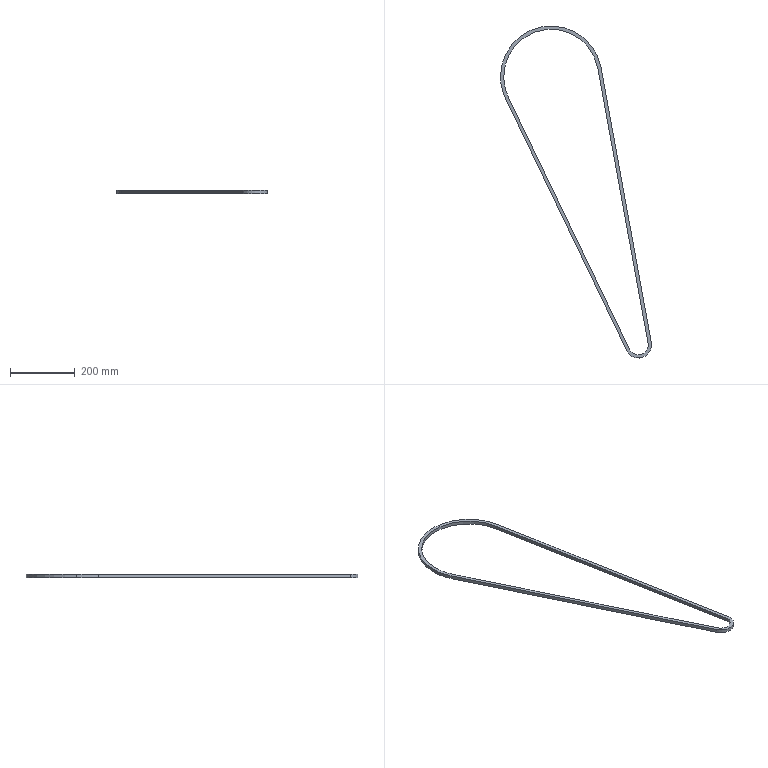Part | SolidWorks | features ExtruThin 1 | 1 solid | 12 faces | box 465.093 x 1023 x 10 mm | volume 233862 mm3 | cylinder 6 | plane 6 | commonest cylinder face diameters 292.108 x2 312.108 x2 60.38 x1 80.38 x1
STEP:
#1=CARTESIAN_POINT('',(143.673,109.871,10.));
#2=VERTEX_POINT('',#1);
#3=CARTESIAN_POINT('',(-146.054,83.608,10.));
#4=VERTEX_POINT('',#3);
#5=CARTESIAN_POINT('',(0.,83.608,10.));
#6=DIRECTION('',(0.,0.,1.));
#7=DIRECTION('',(1.,0.,0.));
#8=AXIS2_PLACEMENT_3D('',#5,#6,#7);
#9=CIRCLE('',#8,146.054);
#10=EDGE_CURVE('',#2,#4,#9,.T.);
#11=ORIENTED_EDGE('',*,*,#10,.T.);
#12=CARTESIAN_POINT('',(-146.054,83.608,0.));
#13=VERTEX_POINT('',#12);
#14=CARTESIAN_POINT('',(-146.054,83.608,10.));
#15=DIRECTION('',(0.,0.,-1.));
#16=VECTOR('',#15,1000.);
#17=LINE('',#14,#16);
#18=EDGE_CURVE('',#4,#13,#17,.T.);
#19=ORIENTED_EDGE('',*,*,#18,.T.);
#20=CARTESIAN_POINT('',(143.673,109.871,0.));
#21=VERTEX_POINT('',#20);
#22=CARTESIAN_POINT('',(0.,83.608,0.));
#23=DIRECTION('',(0.,0.,1.));
#24=DIRECTION('',(1.,0.,0.));
#25=AXIS2_PLACEMENT_3D('',#22,#23,#24);
#26=CIRCLE('',#25,146.054);
#27=EDGE_CURVE('',#21,#13,#26,.T.);
#28=ORIENTED_EDGE('',*,*,#27,.F.);
#29=CARTESIAN_POINT('',(143.673,109.871,10.));
#30=DIRECTION('',(0.,0.,-1.));
#31=VECTOR('',#30,1000.);
#32=LINE('',#29,#31);
#33=EDGE_CURVE('',#2,#21,#32,.T.);
#34=ORIENTED_EDGE('',*,*,#33,.F.);
#35=EDGE_LOOP('',(#11,#19,#28,#34));
#36=FACE_OUTER_BOUND('',#35,.T.);
#37=CARTESIAN_POINT('',(0.,83.608,10.));
#38=DIRECTION('',(0.,0.,-1.));
#39=DIRECTION('',(-1.,0.,0.));
#40=AXIS2_PLACEMENT_3D('',#37,#38,#39);
#41=CYLINDRICAL_SURFACE('',#40,146.054);
#42=ADVANCED_FACE('',(#36),#41,.F.);
#43=CARTESIAN_POINT('',(-156.054,83.608,10.));
#44=VERTEX_POINT('',#43);
#45=CARTESIAN_POINT('',(-140.636,15.975,10.));
#46=VERTEX_POINT('',#45);
#47=CARTESIAN_POINT('',(0.,83.608,10.));
#48=DIRECTION('',(0.,0.,1.));
#49=DIRECTION('',(1.,0.,0.));
#50=AXIS2_PLACEMENT_3D('',#47,#48,#49);
#51=CIRCLE('',#50,156.054);
#52=EDGE_CURVE('',#44,#46,#51,.T.);
#53=ORIENTED_EDGE('',*,*,#52,.F.);
#54=CARTESIAN_POINT('',(-156.054,83.608,0.));
#55=VERTEX_POINT('',#54);
#56=CARTESIAN_POINT('',(-156.054,83.608,10.));
#57=DIRECTION('',(0.,0.,-1.));
#58=VECTOR('',#57,1000.);
#59=LINE('',#56,#58);
#60=EDGE_CURVE('',#44,#55,#59,.T.);
#61=ORIENTED_EDGE('',*,*,#60,.T.);
#62=CARTESIAN_POINT('',(-140.636,15.975,0.));
#63=VERTEX_POINT('',#62);
#64=CARTESIAN_POINT('',(0.,83.608,0.));
#65=DIRECTION('',(0.,0.,1.));
#66=DIRECTION('',(1.,0.,0.));
#67=AXIS2_PLACEMENT_3D('',#64,#65,#66);
#68=CIRCLE('',#67,156.054);
#69=EDGE_CURVE('',#55,#63,#68,.T.);
#70=ORIENTED_EDGE('',*,*,#69,.T.);
#71=CARTESIAN_POINT('',(-140.636,15.975,10.));
#72=DIRECTION('',(0.,0.,-1.));
#73=VECTOR('',#72,1000.);
#74=LINE('',#71,#73);
#75=EDGE_CURVE('',#46,#63,#74,.T.);
#76=ORIENTED_EDGE('',*,*,#75,.F.);
#77=EDGE_LOOP('',(#53,#61,#70,#76));
#78=FACE_OUTER_BOUND('',#77,.T.);
#79=CARTESIAN_POINT('',(0.,83.608,10.));
#80=DIRECTION('',(0.,0.,-1.));
#81=DIRECTION('',(-1.,0.,0.));
#82=AXIS2_PLACEMENT_3D('',#79,#80,#81);
#83=CYLINDRICAL_SURFACE('',#82,156.054);
#84=ADVANCED_FACE('',(#78),#83,.T.);
#85=CARTESIAN_POINT('',(232.63,-760.201,10.));
#86=VERTEX_POINT('',#85);
#87=CARTESIAN_POINT('',(308.384,-735.556,10.));
#88=VERTEX_POINT('',#87);
#89=CARTESIAN_POINT('',(268.849,-742.783,10.));
#90=DIRECTION('',(0.,0.,1.));
#91=DIRECTION('',(1.,0.,0.));
#92=AXIS2_PLACEMENT_3D('',#89,#90,#91);
#93=CIRCLE('',#92,40.19);
#94=EDGE_CURVE('',#86,#88,#93,.T.);
#95=ORIENTED_EDGE('',*,*,#94,.T.);
#96=CARTESIAN_POINT('',(153.51,111.669,10.));
#97=VERTEX_POINT('',#96);
#98=CARTESIAN_POINT('',(153.51,111.669,10.));
#99=DIRECTION('',(-0.1798,0.9837,0.));
#100=VECTOR('',#99,1000.);
#101=LINE('',#98,#100);
#102=EDGE_CURVE('',#88,#97,#101,.T.);
#103=ORIENTED_EDGE('',*,*,#102,.T.);
#104=CARTESIAN_POINT('',(0.,83.608,10.));
#105=DIRECTION('',(0.,0.,1.));
#106=DIRECTION('',(1.,0.,0.));
#107=AXIS2_PLACEMENT_3D('',#104,#105,#106);
#108=CIRCLE('',#107,156.054);
#109=EDGE_CURVE('',#97,#44,#108,.T.);
#110=ORIENTED_EDGE('',*,*,#109,.T.);
#111=ORIENTED_EDGE('',*,*,#52,.T.);
#112=CARTESIAN_POINT('',(-140.636,15.975,10.));
#113=DIRECTION('',(0.4334,-0.9012,0.));
#114=VECTOR('',#113,1000.);
#115=LINE('',#112,#114);
#116=EDGE_CURVE('',#46,#86,#115,.T.);
#117=ORIENTED_EDGE('',*,*,#116,.T.);
#118=EDGE_LOOP('',(#95,#103,#110,#111,#117));
#119=FACE_OUTER_BOUND('',#118,.T.);
#120=CARTESIAN_POINT('',(298.547,-737.354,10.));
#121=VERTEX_POINT('',#120);
#122=CARTESIAN_POINT('',(143.673,109.871,10.));
#123=DIRECTION('',(-0.1798,0.9837,0.));
#124=VECTOR('',#123,1000.);
#125=LINE('',#122,#124);
#126=EDGE_CURVE('',#121,#2,#125,.T.);
#127=ORIENTED_EDGE('',*,*,#126,.F.);
#128=CARTESIAN_POINT('',(241.642,-755.867,10.));
#129=VERTEX_POINT('',#128);
#130=CARTESIAN_POINT('',(268.849,-742.783,10.));
#131=DIRECTION('',(0.,0.,1.));
#132=DIRECTION('',(1.,0.,0.));
#133=AXIS2_PLACEMENT_3D('',#130,#131,#132);
#134=CIRCLE('',#133,30.19);
#135=EDGE_CURVE('',#129,#121,#134,.T.);
#136=ORIENTED_EDGE('',*,*,#135,.F.);
#137=CARTESIAN_POINT('',(-131.624,20.309,10.));
#138=VERTEX_POINT('',#137);
#139=CARTESIAN_POINT('',(-131.624,20.309,10.));
#140=DIRECTION('',(0.4334,-0.9012,0.));
#141=VECTOR('',#140,1000.);
#142=LINE('',#139,#141);
#143=EDGE_CURVE('',#138,#129,#142,.T.);
#144=ORIENTED_EDGE('',*,*,#143,.F.);
#145=CARTESIAN_POINT('',(0.,83.608,10.));
#146=DIRECTION('',(0.,0.,1.));
#147=DIRECTION('',(1.,0.,0.));
#148=AXIS2_PLACEMENT_3D('',#145,#146,#147);
#149=CIRCLE('',#148,146.054);
#150=EDGE_CURVE('',#4,#138,#149,.T.);
#151=ORIENTED_EDGE('',*,*,#150,.F.);
#152=ORIENTED_EDGE('',*,*,#10,.F.);
#153=EDGE_LOOP('',(#127,#136,#144,#151,#152));
#154=FACE_BOUND('',#153,.T.);
#155=CARTESIAN_POINT('',(268.849,-742.783,10.));
#156=DIRECTION('',(0.,0.,1.));
#157=DIRECTION('',(1.,0.,0.));
#158=AXIS2_PLACEMENT_3D('',#155,#156,#157);
#159=PLANE('',#158);
#160=ADVANCED_FACE('',(#119,#154),#159,.T.);
#161=CARTESIAN_POINT('',(232.63,-760.201,0.));
#162=VERTEX_POINT('',#161);
#163=CARTESIAN_POINT('',(308.384,-735.556,0.));
#164=VERTEX_POINT('',#163);
#165=CARTESIAN_POINT('',(268.849,-742.783,0.));
#166=DIRECTION('',(0.,0.,1.));
#167=DIRECTION('',(1.,0.,0.));
#168=AXIS2_PLACEMENT_3D('',#165,#166,#167);
#169=CIRCLE('',#168,40.19);
#170=EDGE_CURVE('',#162,#164,#169,.T.);
#171=ORIENTED_EDGE('',*,*,#170,.F.);
#172=CARTESIAN_POINT('',(-140.636,15.975,0.));
#173=DIRECTION('',(0.4334,-0.9012,0.));
#174=VECTOR('',#173,1000.);
#175=LINE('',#172,#174);
#176=EDGE_CURVE('',#63,#162,#175,.T.);
#177=ORIENTED_EDGE('',*,*,#176,.F.);
#178=ORIENTED_EDGE('',*,*,#69,.F.);
#179=CARTESIAN_POINT('',(153.51,111.669,0.));
#180=VERTEX_POINT('',#179);
#181=CARTESIAN_POINT('',(0.,83.608,0.));
#182=DIRECTION('',(0.,0.,1.));
#183=DIRECTION('',(1.,0.,0.));
#184=AXIS2_PLACEMENT_3D('',#181,#182,#183);
#185=CIRCLE('',#184,156.054);
#186=EDGE_CURVE('',#180,#55,#185,.T.);
#187=ORIENTED_EDGE('',*,*,#186,.F.);
#188=CARTESIAN_POINT('',(153.51,111.669,0.));
#189=DIRECTION('',(-0.1798,0.9837,0.));
#190=VECTOR('',#189,1000.);
#191=LINE('',#188,#190);
#192=EDGE_CURVE('',#164,#180,#191,.T.);
#193=ORIENTED_EDGE('',*,*,#192,.F.);
#194=EDGE_LOOP('',(#171,#177,#178,#187,#193));
#195=FACE_OUTER_BOUND('',#194,.T.);
#196=CARTESIAN_POINT('',(241.642,-755.867,0.));
#197=VERTEX_POINT('',#196);
#198=CARTESIAN_POINT('',(298.547,-737.354,0.));
#199=VERTEX_POINT('',#198);
#200=CARTESIAN_POINT('',(268.849,-742.783,0.));
#201=DIRECTION('',(0.,0.,1.));
#202=DIRECTION('',(1.,0.,0.));
#203=AXIS2_PLACEMENT_3D('',#200,#201,#202);
#204=CIRCLE('',#203,30.19);
#205=EDGE_CURVE('',#197,#199,#204,.T.);
#206=ORIENTED_EDGE('',*,*,#205,.T.);
#207=CARTESIAN_POINT('',(143.673,109.871,0.));
#208=DIRECTION('',(-0.1798,0.9837,0.));
#209=VECTOR('',#208,1000.);
#210=LINE('',#207,#209);
#211=EDGE_CURVE('',#199,#21,#210,.T.);
#212=ORIENTED_EDGE('',*,*,#211,.T.);
#213=ORIENTED_EDGE('',*,*,#27,.T.);
#214=CARTESIAN_POINT('',(-131.624,20.309,0.));
#215=VERTEX_POINT('',#214);
#216=CARTESIAN_POINT('',(0.,83.608,0.));
#217=DIRECTION('',(0.,0.,1.));
#218=DIRECTION('',(1.,0.,0.));
#219=AXIS2_PLACEMENT_3D('',#216,#217,#218);
#220=CIRCLE('',#219,146.054);
#221=EDGE_CURVE('',#13,#215,#220,.T.);
#222=ORIENTED_EDGE('',*,*,#221,.T.);
#223=CARTESIAN_POINT('',(-131.624,20.309,0.));
#224=DIRECTION('',(0.4334,-0.9012,0.));
#225=VECTOR('',#224,1000.);
#226=LINE('',#223,#225);
#227=EDGE_CURVE('',#215,#197,#226,.T.);
#228=ORIENTED_EDGE('',*,*,#227,.T.);
#229=EDGE_LOOP('',(#206,#212,#213,#222,#228));
#230=FACE_BOUND('',#229,.T.);
#231=CARTESIAN_POINT('',(268.849,-742.783,0.));
#232=DIRECTION('',(0.,0.,1.));
#233=DIRECTION('',(1.,0.,0.));
#234=AXIS2_PLACEMENT_3D('',#231,#232,#233);
#235=PLANE('',#234);
#236=ADVANCED_FACE('',(#195,#230),#235,.F.);
#237=ORIENTED_EDGE('',*,*,#170,.T.);
#238=CARTESIAN_POINT('',(308.384,-735.556,10.));
#239=DIRECTION('',(0.,0.,-1.));
#240=VECTOR('',#239,1000.);
#241=LINE('',#238,#240);
#242=EDGE_CURVE('',#88,#164,#241,.T.);
#243=ORIENTED_EDGE('',*,*,#242,.F.);
#244=ORIENTED_EDGE('',*,*,#94,.F.);
#245=CARTESIAN_POINT('',(232.63,-760.201,10.));
#246=DIRECTION('',(0.,0.,-1.));
#247=VECTOR('',#246,1000.);
#248=LINE('',#245,#247);
#249=EDGE_CURVE('',#86,#162,#248,.T.);
#250=ORIENTED_EDGE('',*,*,#249,.T.);
#251=EDGE_LOOP('',(#237,#243,#244,#250));
#252=FACE_OUTER_BOUND('',#251,.T.);
#253=CARTESIAN_POINT('',(268.849,-742.783,10.));
#254=DIRECTION('',(0.,0.,-1.));
#255=DIRECTION('',(-1.,0.,0.));
#256=AXIS2_PLACEMENT_3D('',#253,#254,#255);
#257=CYLINDRICAL_SURFACE('',#256,40.19);
#258=ADVANCED_FACE('',(#252),#257,.T.);
#259=ORIENTED_EDGE('',*,*,#192,.T.);
#260=CARTESIAN_POINT('',(153.51,111.669,10.));
#261=DIRECTION('',(0.,0.,-1.));
#262=VECTOR('',#261,1000.);
#263=LINE('',#260,#262);
#264=EDGE_CURVE('',#97,#180,#263,.T.);
#265=ORIENTED_EDGE('',*,*,#264,.F.);
#266=ORIENTED_EDGE('',*,*,#102,.F.);
#267=ORIENTED_EDGE('',*,*,#242,.T.);
#268=EDGE_LOOP('',(#259,#265,#266,#267));
#269=FACE_OUTER_BOUND('',#268,.T.);
#270=CARTESIAN_POINT('',(153.51,111.669,10.));
#271=DIRECTION('',(-0.9837,-0.1798,0.));
#272=DIRECTION('',(0.1798,-0.9837,0.));
#273=AXIS2_PLACEMENT_3D('',#270,#271,#272);
#274=PLANE('',#273);
#275=ADVANCED_FACE('',(#269),#274,.F.);
#276=ORIENTED_EDGE('',*,*,#60,.F.);
#277=ORIENTED_EDGE('',*,*,#109,.F.);
#278=ORIENTED_EDGE('',*,*,#264,.T.);
#279=ORIENTED_EDGE('',*,*,#186,.T.);
#280=EDGE_LOOP('',(#276,#277,#278,#279));
#281=FACE_OUTER_BOUND('',#280,.T.);
#282=CARTESIAN_POINT('',(0.,83.608,10.));
#283=DIRECTION('',(0.,0.,-1.));
#284=DIRECTION('',(-1.,0.,0.));
#285=AXIS2_PLACEMENT_3D('',#282,#283,#284);
#286=CYLINDRICAL_SURFACE('',#285,156.054);
#287=ADVANCED_FACE('',(#281),#286,.T.);
#288=ORIENTED_EDGE('',*,*,#176,.T.);
#289=ORIENTED_EDGE('',*,*,#249,.F.);
#290=ORIENTED_EDGE('',*,*,#116,.F.);
#291=ORIENTED_EDGE('',*,*,#75,.T.);
#292=EDGE_LOOP('',(#288,#289,#290,#291));
#293=FACE_OUTER_BOUND('',#292,.T.);
#294=CARTESIAN_POINT('',(-140.636,15.975,10.));
#295=DIRECTION('',(0.9012,0.4334,0.));
#296=DIRECTION('',(-0.4334,0.9012,0.));
#297=AXIS2_PLACEMENT_3D('',#294,#295,#296);
#298=PLANE('',#297);
#299=ADVANCED_FACE('',(#293),#298,.F.);
#300=ORIENTED_EDGE('',*,*,#205,.F.);
#301=CARTESIAN_POINT('',(241.642,-755.867,10.));
#302=DIRECTION('',(0.,0.,-1.));
#303=VECTOR('',#302,1000.);
#304=LINE('',#301,#303);
#305=EDGE_CURVE('',#129,#197,#304,.T.);
#306=ORIENTED_EDGE('',*,*,#305,.F.);
#307=ORIENTED_EDGE('',*,*,#135,.T.);
#308=CARTESIAN_POINT('',(298.547,-737.354,10.));
#309=DIRECTION('',(0.,0.,-1.));
#310=VECTOR('',#309,1000.);
#311=LINE('',#308,#310);
#312=EDGE_CURVE('',#121,#199,#311,.T.);
#313=ORIENTED_EDGE('',*,*,#312,.T.);
#314=EDGE_LOOP('',(#300,#306,#307,#313));
#315=FACE_OUTER_BOUND('',#314,.T.);
#316=CARTESIAN_POINT('',(268.849,-742.783,10.));
#317=DIRECTION('',(0.,0.,-1.));
#318=DIRECTION('',(-1.,0.,0.));
#319=AXIS2_PLACEMENT_3D('',#316,#317,#318);
#320=CYLINDRICAL_SURFACE('',#319,30.19);
#321=ADVANCED_FACE('',(#315),#320,.F.);
#322=ORIENTED_EDGE('',*,*,#211,.F.);
#323=ORIENTED_EDGE('',*,*,#312,.F.);
#324=ORIENTED_EDGE('',*,*,#126,.T.);
#325=ORIENTED_EDGE('',*,*,#33,.T.);
#326=EDGE_LOOP('',(#322,#323,#324,#325));
#327=FACE_OUTER_BOUND('',#326,.T.);
#328=CARTESIAN_POINT('',(143.673,109.871,10.));
#329=DIRECTION('',(-0.9837,-0.1798,0.));
#330=DIRECTION('',(0.1798,-0.9837,0.));
#331=AXIS2_PLACEMENT_3D('',#328,#329,#330);
#332=PLANE('',#331);
#333=ADVANCED_FACE('',(#327),#332,.T.);
#334=ORIENTED_EDGE('',*,*,#18,.F.);
#335=ORIENTED_EDGE('',*,*,#150,.T.);
#336=CARTESIAN_POINT('',(-131.624,20.309,10.));
#337=DIRECTION('',(0.,0.,-1.));
#338=VECTOR('',#337,1000.);
#339=LINE('',#336,#338);
#340=EDGE_CURVE('',#138,#215,#339,.T.);
#341=ORIENTED_EDGE('',*,*,#340,.T.);
#342=ORIENTED_EDGE('',*,*,#221,.F.);
#343=EDGE_LOOP('',(#334,#335,#341,#342));
#344=FACE_OUTER_BOUND('',#343,.T.);
#345=CARTESIAN_POINT('',(0.,83.608,10.));
#346=DIRECTION('',(0.,0.,-1.));
#347=DIRECTION('',(-1.,0.,0.));
#348=AXIS2_PLACEMENT_3D('',#345,#346,#347);
#349=CYLINDRICAL_SURFACE('',#348,146.054);
#350=ADVANCED_FACE('',(#344),#349,.F.);
#351=ORIENTED_EDGE('',*,*,#227,.F.);
#352=ORIENTED_EDGE('',*,*,#340,.F.);
#353=ORIENTED_EDGE('',*,*,#143,.T.);
#354=ORIENTED_EDGE('',*,*,#305,.T.);
#355=EDGE_LOOP('',(#351,#352,#353,#354));
#356=FACE_OUTER_BOUND('',#355,.T.);
#357=CARTESIAN_POINT('',(-131.624,20.309,10.));
#358=DIRECTION('',(0.9012,0.4334,0.));
#359=DIRECTION('',(-0.4334,0.9012,0.));
#360=AXIS2_PLACEMENT_3D('',#357,#358,#359);
#361=PLANE('',#360);
#362=ADVANCED_FACE('',(#356),#361,.T.);
#363=CLOSED_SHELL('',(#42,#84,#160,#236,#258,#275,#287,#299,#321,#333,#350,#362));
#364=MANIFOLD_SOLID_BREP('',#363);
#365=CARTESIAN_POINT('',(0.,0.,0.));
#366=DIRECTION('',(0.,0.,1.));
#367=DIRECTION('',(1.,0.,0.));
#368=AXIS2_PLACEMENT_3D('',#365,#366,#367);
#369=(LENGTH_UNIT()NAMED_UNIT(*)SI_UNIT(.MILLI.,.METRE.));
#370=UNCERTAINTY_MEASURE_WITH_UNIT(LENGTH_MEASURE(0.00001),#369,'','');
#371=(NAMED_UNIT(*)PLANE_ANGLE_UNIT()SI_UNIT($,.RADIAN.));
#372=(NAMED_UNIT(*)SI_UNIT($,.STERADIAN.)SOLID_ANGLE_UNIT());
#373=(GEOMETRIC_REPRESENTATION_CONTEXT(3)GLOBAL_UNCERTAINTY_ASSIGNED_CONTEXT((#370))GLOBAL_UNIT_ASSIGNED_CONTEXT((#369,#371,#372))REPRESENTATION_CONTEXT('',''));
#374=ADVANCED_BREP_SHAPE_REPRESENTATION('',(#364,#368),#373);